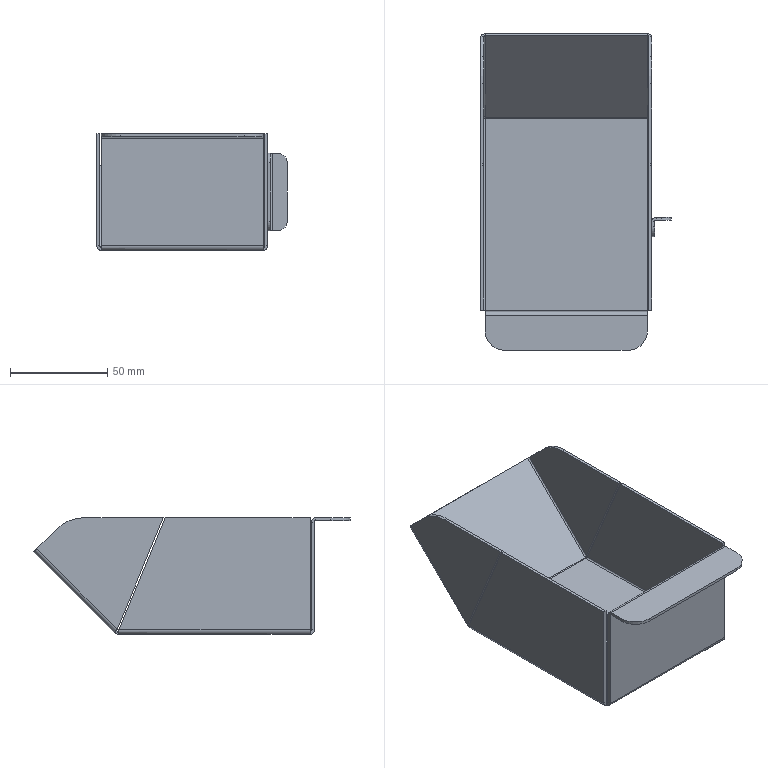Part | STEP file | 08-24 recheck collection box (Default_as machined_) | 2 solids | 88 faces | box 98 x 163.048 x 60 mm | volume 52980 mm3 | plane 56 | cylinder 24 | spline 8 | commonest cylinder face diameters 1.473 x8 4.473 x8 10 x4 20 x2 40 x2